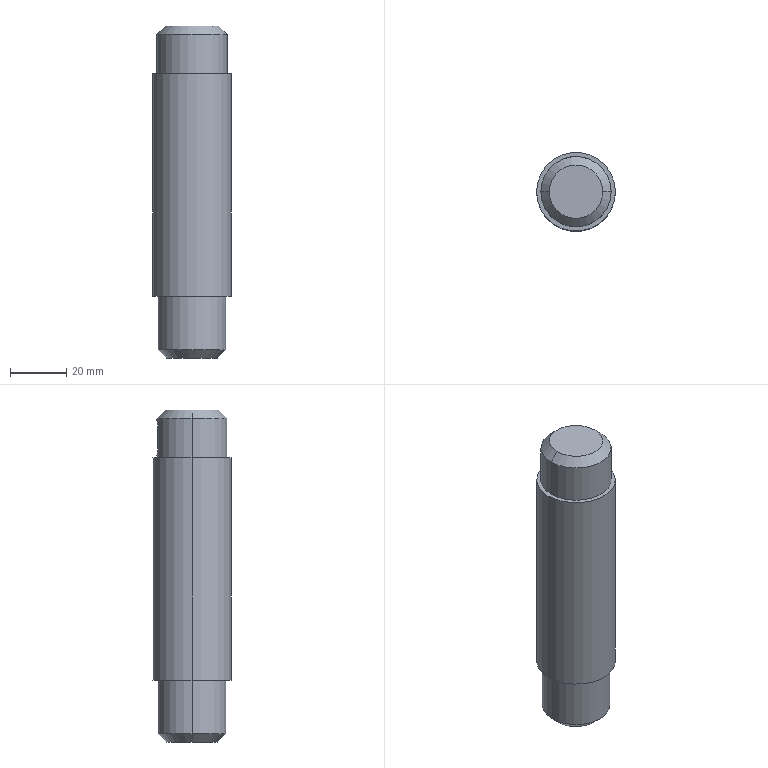Part | SolidWorks | features ICE 2, Chamfer 1, Cut 1, Extrusion 1, MoveFace 1 | 1 solid | 20 faces | box 28 x 28 x 118 mm | volume 66131 mm3 | cylinder 9 | plane 7 | cone 4 | commonest cylinder face diameters 5 x3 24 x2 25 x2 28 x2
STEP:
#1=CARTESIAN_POINT('',(0.,9.5,92.7));
#2=VERTEX_POINT('',#1);
#3=CARTESIAN_POINT('',(2.5,9.5,90.2));
#4=VERTEX_POINT('',#3);
#5=CARTESIAN_POINT('',(0.,9.5,90.2));
#6=DIRECTION('',(0.,1.,0.));
#7=DIRECTION('',(0.,0.,1.));
#8=AXIS2_PLACEMENT_3D('',#5,#6,#7);
#9=CIRCLE('',#8,2.5);
#10=EDGE_CURVE('',#2,#4,#9,.T.);
#11=ORIENTED_EDGE('',*,*,#10,.F.);
#12=CARTESIAN_POINT('',(0.,12.5,92.7));
#13=VERTEX_POINT('',#12);
#14=CARTESIAN_POINT('',(0.,9.5,92.7));
#15=DIRECTION('',(0.,1.,0.));
#16=VECTOR('',#15,1000.);
#17=LINE('',#14,#16);
#18=EDGE_CURVE('',#2,#13,#17,.T.);
#19=ORIENTED_EDGE('',*,*,#18,.T.);
#20=CARTESIAN_POINT('',(2.5,12.247,90.2));
#21=VERTEX_POINT('',#20);
#22=CARTESIAN_POINT('',(0.,12.5,92.7));
#23=CARTESIAN_POINT('',(0.1634,12.5,92.7));
#24=CARTESIAN_POINT('',(0.3294,12.497,92.684));
#25=CARTESIAN_POINT('',(0.6501,12.484,92.62));
#26=CARTESIAN_POINT('',(0.806,12.475,92.572));
#27=CARTESIAN_POINT('',(1.109,12.452,92.447));
#28=CARTESIAN_POINT('',(1.255,12.438,92.368));
#29=CARTESIAN_POINT('',(1.525,12.407,92.188));
#30=CARTESIAN_POINT('',(1.651,12.391,92.084));
#31=CARTESIAN_POINT('',(1.884,12.358,91.852));
#32=CARTESIAN_POINT('',(1.987,12.341,91.726));
#33=CARTESIAN_POINT('',(2.168,12.311,91.456));
#34=CARTESIAN_POINT('',(2.246,12.297,91.31));
#35=CARTESIAN_POINT('',(2.371,12.273,91.008));
#36=CARTESIAN_POINT('',(2.419,12.264,90.852));
#37=CARTESIAN_POINT('',(2.483,12.251,90.531));
#38=CARTESIAN_POINT('',(2.5,12.247,90.366));
#39=CARTESIAN_POINT('',(2.5,12.247,90.2));
#40=B_SPLINE_CURVE_WITH_KNOTS('',3,(#22,#23,#24,#25,#26,#27,#28,#29,#30,#31,#32,#33,#34,#35,#36,#37,#38,#39),.UNSPECIFIED.,.F.,.F.,(4,2,2,2,2,2,2,2,4),(0.003919,0.004408,0.004898,0.005387,0.005876,0.006366,0.006855,0.007344,0.007834),.UNSPECIFIED.);
#41=EDGE_CURVE('',#13,#21,#40,.T.);
#42=ORIENTED_EDGE('',*,*,#41,.T.);
#43=CARTESIAN_POINT('',(2.5,9.5,90.2));
#44=DIRECTION('',(0.,1.,0.));
#45=VECTOR('',#44,1000.);
#46=LINE('',#43,#45);
#47=EDGE_CURVE('',#4,#21,#46,.T.);
#48=ORIENTED_EDGE('',*,*,#47,.F.);
#49=EDGE_LOOP('',(#11,#19,#42,#48));
#50=FACE_OUTER_BOUND('',#49,.T.);
#51=CARTESIAN_POINT('',(0.,9.5,90.2));
#52=DIRECTION('',(0.,1.,0.));
#53=DIRECTION('',(0.,0.,1.));
#54=AXIS2_PLACEMENT_3D('',#51,#52,#53);
#55=CYLINDRICAL_SURFACE('',#54,2.5);
#56=ADVANCED_FACE('',(#50),#55,.F.);
#57=CARTESIAN_POINT('',(9.5,0.,96.));
#58=VERTEX_POINT('',#57);
#59=CARTESIAN_POINT('',(-9.5,0.,96.));
#60=VERTEX_POINT('',#59);
#61=CARTESIAN_POINT('',(0.,0.,96.));
#62=DIRECTION('',(0.,0.,1.));
#63=DIRECTION('',(1.,0.,0.));
#64=AXIS2_PLACEMENT_3D('',#61,#62,#63);
#65=CIRCLE('',#64,9.5);
#66=EDGE_CURVE('',#58,#60,#65,.T.);
#67=ORIENTED_EDGE('',*,*,#66,.F.);
#68=CARTESIAN_POINT('',(12.5,0.,93.));
#69=VERTEX_POINT('',#68);
#70=CARTESIAN_POINT('',(9.5,0.,96.));
#71=DIRECTION('',(0.7071,0.,-0.7071));
#72=VECTOR('',#71,1000.);
#73=LINE('',#70,#72);
#74=EDGE_CURVE('',#58,#69,#73,.T.);
#75=ORIENTED_EDGE('',*,*,#74,.T.);
#76=CARTESIAN_POINT('',(-12.5,0.,93.));
#77=VERTEX_POINT('',#76);
#78=CARTESIAN_POINT('',(0.,0.,93.));
#79=DIRECTION('',(0.,0.,-1.));
#80=DIRECTION('',(1.,0.,0.));
#81=AXIS2_PLACEMENT_3D('',#78,#79,#80);
#82=CIRCLE('',#81,12.5);
#83=EDGE_CURVE('',#77,#69,#82,.T.);
#84=ORIENTED_EDGE('',*,*,#83,.F.);
#85=CARTESIAN_POINT('',(-9.5,0.,96.));
#86=DIRECTION('',(-0.7071,0.,-0.7071));
#87=VECTOR('',#86,1000.);
#88=LINE('',#85,#87);
#89=EDGE_CURVE('',#60,#77,#88,.T.);
#90=ORIENTED_EDGE('',*,*,#89,.F.);
#91=EDGE_LOOP('',(#67,#75,#84,#90));
#92=FACE_OUTER_BOUND('',#91,.T.);
#93=CARTESIAN_POINT('',(0.,0.,96.));
#94=DIRECTION('',(0.,0.,-1.));
#95=DIRECTION('',(-1.,0.,0.));
#96=AXIS2_PLACEMENT_3D('',#93,#94,#95);
#97=CONICAL_SURFACE('',#96,9.5,0.7854);
#98=ADVANCED_FACE('',(#92),#97,.T.);
#99=CARTESIAN_POINT('',(-9.,0.,-22.));
#100=VERTEX_POINT('',#99);
#101=CARTESIAN_POINT('',(9.,0.,-22.));
#102=VERTEX_POINT('',#101);
#103=CARTESIAN_POINT('',(0.,0.,-22.));
#104=DIRECTION('',(0.,0.,-1.));
#105=DIRECTION('',(1.,0.,0.));
#106=AXIS2_PLACEMENT_3D('',#103,#104,#105);
#107=CIRCLE('',#106,9.);
#108=EDGE_CURVE('',#100,#102,#107,.T.);
#109=ORIENTED_EDGE('',*,*,#108,.F.);
#110=CARTESIAN_POINT('',(-12.,0.,-19.));
#111=VERTEX_POINT('',#110);
#112=CARTESIAN_POINT('',(-12.,0.,-19.));
#113=DIRECTION('',(-0.7071,0.,0.7071));
#114=VECTOR('',#113,1000.);
#115=LINE('',#112,#114);
#116=EDGE_CURVE('',#100,#111,#115,.T.);
#117=ORIENTED_EDGE('',*,*,#116,.T.);
#118=CARTESIAN_POINT('',(12.,0.,-19.));
#119=VERTEX_POINT('',#118);
#120=CARTESIAN_POINT('',(0.,0.,-19.));
#121=DIRECTION('',(0.,0.,1.));
#122=DIRECTION('',(1.,0.,0.));
#123=AXIS2_PLACEMENT_3D('',#120,#121,#122);
#124=CIRCLE('',#123,12.);
#125=EDGE_CURVE('',#119,#111,#124,.T.);
#126=ORIENTED_EDGE('',*,*,#125,.F.);
#127=CARTESIAN_POINT('',(12.,0.,-19.));
#128=DIRECTION('',(0.7071,0.,0.7071));
#129=VECTOR('',#128,1000.);
#130=LINE('',#127,#129);
#131=EDGE_CURVE('',#102,#119,#130,.T.);
#132=ORIENTED_EDGE('',*,*,#131,.F.);
#133=EDGE_LOOP('',(#109,#117,#126,#132));
#134=FACE_OUTER_BOUND('',#133,.T.);
#135=CARTESIAN_POINT('',(0.,0.,-19.));
#136=DIRECTION('',(0.,0.,1.));
#137=DIRECTION('',(1.,0.,0.));
#138=AXIS2_PLACEMENT_3D('',#135,#136,#137);
#139=CONICAL_SURFACE('',#138,12.,0.7854);
#140=ADVANCED_FACE('',(#134),#139,.T.);
#141=CARTESIAN_POINT('',(2.5,12.247,82.2));
#142=VERTEX_POINT('',#141);
#143=CARTESIAN_POINT('',(-2.5,12.247,82.2));
#144=VERTEX_POINT('',#143);
#145=CARTESIAN_POINT('',(2.5,12.247,82.2));
#146=CARTESIAN_POINT('',(2.5,12.247,82.034));
#147=CARTESIAN_POINT('',(2.484,12.251,81.872));
#148=CARTESIAN_POINT('',(2.42,12.264,81.552));
#149=CARTESIAN_POINT('',(2.372,12.273,81.393));
#150=CARTESIAN_POINT('',(2.246,12.297,81.09));
#151=CARTESIAN_POINT('',(2.169,12.311,80.947));
#152=CARTESIAN_POINT('',(1.988,12.341,80.675));
#153=CARTESIAN_POINT('',(1.883,12.358,80.547));
#154=CARTESIAN_POINT('',(1.538,12.407,80.202));
#155=CARTESIAN_POINT('',(1.26,12.44,80.016));
#156=CARTESIAN_POINT('',(0.8088,12.475,79.829));
#157=CARTESIAN_POINT('',(0.6508,12.484,79.781));
#158=CARTESIAN_POINT('',(0.328,12.497,79.716));
#159=CARTESIAN_POINT('',(0.1655,12.5,79.7));
#160=CARTESIAN_POINT('',(-0.1614,12.5,79.7));
#161=CARTESIAN_POINT('',(-0.3276,12.497,79.716));
#162=CARTESIAN_POINT('',(-0.6485,12.484,79.78));
#163=CARTESIAN_POINT('',(-0.8045,12.475,79.827));
#164=CARTESIAN_POINT('',(-1.108,12.452,79.953));
#165=CARTESIAN_POINT('',(-1.253,12.438,80.031));
#166=CARTESIAN_POINT('',(-1.524,12.408,80.211));
#167=CARTESIAN_POINT('',(-1.651,12.391,80.315));
#168=CARTESIAN_POINT('',(-1.883,12.358,80.547));
#169=CARTESIAN_POINT('',(-1.986,12.342,80.673));
#170=CARTESIAN_POINT('',(-2.167,12.311,80.943));
#171=CARTESIAN_POINT('',(-2.246,12.297,81.09));
#172=CARTESIAN_POINT('',(-2.371,12.273,81.392));
#173=CARTESIAN_POINT('',(-2.419,12.264,81.547));
#174=CARTESIAN_POINT('',(-2.483,12.251,81.869));
#175=CARTESIAN_POINT('',(-2.5,12.247,82.034));
#176=CARTESIAN_POINT('',(-2.5,12.247,82.2));
#177=B_SPLINE_CURVE_WITH_KNOTS('',3,(#145,#146,#147,#148,#149,#150,#151,#152,#153,#154,#155,#156,#157,#158,#159,#160,#161,#162,#163,#164,#165,#166,#167,#168,#169,#170,#171,#172,#173,#174,#175,#176),.UNSPECIFIED.,.F.,.F.,(4,2,2,2,2,2,2,2,2,2,2,2,2,2,2,4),(0.,0.0004896,0.0009792,0.001469,0.001958,0.002938,0.003427,0.003917,0.004407,0.004896,0.005386,0.005875,0.006365,0.006855,0.007344,0.007834),.UNSPECIFIED.);
#178=EDGE_CURVE('',#142,#144,#177,.T.);
#179=ORIENTED_EDGE('',*,*,#178,.F.);
#180=CARTESIAN_POINT('',(2.5,12.247,30.));
#181=DIRECTION('',(0.,0.,-1.));
#182=VECTOR('',#181,1000.);
#183=LINE('',#180,#182);
#184=EDGE_CURVE('',#21,#142,#183,.T.);
#185=ORIENTED_EDGE('',*,*,#184,.F.);
#186=ORIENTED_EDGE('',*,*,#41,.F.);
#187=CARTESIAN_POINT('',(-2.5,12.247,90.2));
#188=VERTEX_POINT('',#187);
#189=CARTESIAN_POINT('',(-2.5,12.247,90.2));
#190=CARTESIAN_POINT('',(-2.5,12.247,90.366));
#191=CARTESIAN_POINT('',(-2.484,12.251,90.528));
#192=CARTESIAN_POINT('',(-2.42,12.264,90.849));
#193=CARTESIAN_POINT('',(-2.372,12.273,91.008));
#194=CARTESIAN_POINT('',(-2.246,12.297,91.31));
#195=CARTESIAN_POINT('',(-2.169,12.311,91.454));
#196=CARTESIAN_POINT('',(-1.987,12.341,91.725));
#197=CARTESIAN_POINT('',(-1.882,12.358,91.854));
#198=CARTESIAN_POINT('',(-1.537,12.407,92.198));
#199=CARTESIAN_POINT('',(-1.258,12.44,92.385));
#200=CARTESIAN_POINT('',(-0.8073,12.475,92.572));
#201=CARTESIAN_POINT('',(-0.6491,12.484,92.62));
#202=CARTESIAN_POINT('',(-0.3261,12.497,92.684));
#203=CARTESIAN_POINT('',(-0.1636,12.5,92.7));
#204=CARTESIAN_POINT('',(0.,12.5,92.7));
#205=B_SPLINE_CURVE_WITH_KNOTS('',3,(#189,#190,#191,#192,#193,#194,#195,#196,#197,#198,#199,#200,#201,#202,#203,#204),.UNSPECIFIED.,.F.,.F.,(4,2,2,2,2,2,2,4),(0.,0.0004899,0.0009797,0.00147,0.001959,0.002939,0.003429,0.003919),.UNSPECIFIED.);
#206=EDGE_CURVE('',#188,#13,#205,.T.);
#207=ORIENTED_EDGE('',*,*,#206,.F.);
#208=CARTESIAN_POINT('',(-2.5,12.247,30.));
#209=DIRECTION('',(0.,0.,1.));
#210=VECTOR('',#209,1000.);
#211=LINE('',#208,#210);
#212=EDGE_CURVE('',#144,#188,#211,.T.);
#213=ORIENTED_EDGE('',*,*,#212,.F.);
#214=EDGE_LOOP('',(#179,#185,#186,#207,#213));
#215=FACE_BOUND('',#214,.T.);
#216=CARTESIAN_POINT('',(12.5,0.,79.));
#217=VERTEX_POINT('',#216);
#218=CARTESIAN_POINT('',(-12.5,0.,79.));
#219=VERTEX_POINT('',#218);
#220=CARTESIAN_POINT('',(0.,0.,79.));
#221=DIRECTION('',(0.,0.,1.));
#222=DIRECTION('',(1.,0.,0.));
#223=AXIS2_PLACEMENT_3D('',#220,#221,#222);
#224=CIRCLE('',#223,12.5);
#225=EDGE_CURVE('',#217,#219,#224,.T.);
#226=ORIENTED_EDGE('',*,*,#225,.T.);
#227=CARTESIAN_POINT('',(-12.5,0.,30.));
#228=DIRECTION('',(0.,0.,1.));
#229=VECTOR('',#228,1000.);
#230=LINE('',#227,#229);
#231=EDGE_CURVE('',#219,#77,#230,.T.);
#232=ORIENTED_EDGE('',*,*,#231,.T.);
#233=ORIENTED_EDGE('',*,*,#83,.T.);
#234=CARTESIAN_POINT('',(12.5,0.,30.));
#235=DIRECTION('',(0.,0.,1.));
#236=VECTOR('',#235,1000.);
#237=LINE('',#234,#236);
#238=EDGE_CURVE('',#217,#69,#237,.T.);
#239=ORIENTED_EDGE('',*,*,#238,.F.);
#240=EDGE_LOOP('',(#226,#232,#233,#239));
#241=FACE_OUTER_BOUND('',#240,.T.);
#242=CARTESIAN_POINT('',(0.,0.,30.));
#243=DIRECTION('',(0.,0.,1.));
#244=DIRECTION('',(1.,0.,0.));
#245=AXIS2_PLACEMENT_3D('',#242,#243,#244);
#246=CYLINDRICAL_SURFACE('',#245,12.5);
#247=ADVANCED_FACE('',(#215,#241),#246,.T.);
#248=ORIENTED_EDGE('',*,*,#125,.T.);
#249=CARTESIAN_POINT('',(-12.,0.,0.));
#250=VERTEX_POINT('',#249);
#251=CARTESIAN_POINT('',(-12.,0.,-22.));
#252=DIRECTION('',(0.,0.,1.));
#253=VECTOR('',#252,1000.);
#254=LINE('',#251,#253);
#255=EDGE_CURVE('',#111,#250,#254,.T.);
#256=ORIENTED_EDGE('',*,*,#255,.T.);
#257=CARTESIAN_POINT('',(12.,0.,0.));
#258=VERTEX_POINT('',#257);
#259=CARTESIAN_POINT('',(0.,0.,0.));
#260=DIRECTION('',(0.,0.,1.));
#261=DIRECTION('',(1.,0.,0.));
#262=AXIS2_PLACEMENT_3D('',#259,#260,#261);
#263=CIRCLE('',#262,12.);
#264=EDGE_CURVE('',#258,#250,#263,.T.);
#265=ORIENTED_EDGE('',*,*,#264,.F.);
#266=CARTESIAN_POINT('',(12.,0.,-22.));
#267=DIRECTION('',(0.,0.,1.));
#268=VECTOR('',#267,1000.);
#269=LINE('',#266,#268);
#270=EDGE_CURVE('',#119,#258,#269,.T.);
#271=ORIENTED_EDGE('',*,*,#270,.F.);
#272=EDGE_LOOP('',(#248,#256,#265,#271));
#273=FACE_OUTER_BOUND('',#272,.T.);
#274=CARTESIAN_POINT('',(0.,0.,-22.));
#275=DIRECTION('',(0.,0.,1.));
#276=DIRECTION('',(1.,0.,0.));
#277=AXIS2_PLACEMENT_3D('',#274,#275,#276);
#278=CYLINDRICAL_SURFACE('',#277,12.);
#279=ADVANCED_FACE('',(#273),#278,.T.);
#280=CARTESIAN_POINT('',(14.,0.,79.));
#281=VERTEX_POINT('',#280);
#282=CARTESIAN_POINT('',(-14.,0.,79.));
#283=VERTEX_POINT('',#282);
#284=CARTESIAN_POINT('',(0.,0.,79.));
#285=DIRECTION('',(0.,0.,1.));
#286=DIRECTION('',(1.,0.,0.));
#287=AXIS2_PLACEMENT_3D('',#284,#285,#286);
#288=CIRCLE('',#287,14.);
#289=EDGE_CURVE('',#281,#283,#288,.T.);
#290=ORIENTED_EDGE('',*,*,#289,.F.);
#291=CARTESIAN_POINT('',(14.,0.,0.));
#292=VERTEX_POINT('',#291);
#293=CARTESIAN_POINT('',(14.,0.,96.));
#294=DIRECTION('',(0.,0.,-1.));
#295=VECTOR('',#294,1000.);
#296=LINE('',#293,#295);
#297=EDGE_CURVE('',#281,#292,#296,.T.);
#298=ORIENTED_EDGE('',*,*,#297,.T.);
#299=CARTESIAN_POINT('',(-14.,0.,0.));
#300=VERTEX_POINT('',#299);
#301=CARTESIAN_POINT('',(0.,0.,0.));
#302=DIRECTION('',(0.,0.,1.));
#303=DIRECTION('',(1.,0.,0.));
#304=AXIS2_PLACEMENT_3D('',#301,#302,#303);
#305=CIRCLE('',#304,14.);
#306=EDGE_CURVE('',#292,#300,#305,.T.);
#307=ORIENTED_EDGE('',*,*,#306,.T.);
#308=CARTESIAN_POINT('',(-14.,0.,96.));
#309=DIRECTION('',(0.,0.,-1.));
#310=VECTOR('',#309,1000.);
#311=LINE('',#308,#310);
#312=EDGE_CURVE('',#283,#300,#311,.T.);
#313=ORIENTED_EDGE('',*,*,#312,.F.);
#314=EDGE_LOOP('',(#290,#298,#307,#313));
#315=FACE_OUTER_BOUND('',#314,.T.);
#316=CARTESIAN_POINT('',(0.,0.,96.));
#317=DIRECTION('',(0.,0.,-1.));
#318=DIRECTION('',(-1.,0.,0.));
#319=AXIS2_PLACEMENT_3D('',#316,#317,#318);
#320=CYLINDRICAL_SURFACE('',#319,14.);
#321=ADVANCED_FACE('',(#315),#320,.T.);
#322=ORIENTED_EDGE('',*,*,#297,.F.);
#323=CARTESIAN_POINT('',(0.,0.,79.));
#324=DIRECTION('',(0.,0.,1.));
#325=DIRECTION('',(1.,0.,0.));
#326=AXIS2_PLACEMENT_3D('',#323,#324,#325);
#327=CIRCLE('',#326,14.);
#328=EDGE_CURVE('',#283,#281,#327,.T.);
#329=ORIENTED_EDGE('',*,*,#328,.F.);
#330=ORIENTED_EDGE('',*,*,#312,.T.);
#331=CARTESIAN_POINT('',(0.,0.,0.));
#332=DIRECTION('',(0.,0.,1.));
#333=DIRECTION('',(1.,0.,0.));
#334=AXIS2_PLACEMENT_3D('',#331,#332,#333);
#335=CIRCLE('',#334,14.);
#336=EDGE_CURVE('',#300,#292,#335,.T.);
#337=ORIENTED_EDGE('',*,*,#336,.T.);
#338=EDGE_LOOP('',(#322,#329,#330,#337));
#339=FACE_OUTER_BOUND('',#338,.T.);
#340=CARTESIAN_POINT('',(0.,0.,96.));
#341=DIRECTION('',(0.,0.,-1.));
#342=DIRECTION('',(-1.,0.,0.));
#343=AXIS2_PLACEMENT_3D('',#340,#341,#342);
#344=CYLINDRICAL_SURFACE('',#343,14.);
#345=ADVANCED_FACE('',(#339),#344,.T.);
#346=ORIENTED_EDGE('',*,*,#255,.F.);
#347=CARTESIAN_POINT('',(0.,0.,-19.));
#348=DIRECTION('',(0.,0.,1.));
#349=DIRECTION('',(1.,0.,0.));
#350=AXIS2_PLACEMENT_3D('',#347,#348,#349);
#351=CIRCLE('',#350,12.);
#352=EDGE_CURVE('',#111,#119,#351,.T.);
#353=ORIENTED_EDGE('',*,*,#352,.T.);
#354=ORIENTED_EDGE('',*,*,#270,.T.);
#355=CARTESIAN_POINT('',(0.,0.,0.));
#356=DIRECTION('',(0.,0.,1.));
#357=DIRECTION('',(1.,0.,0.));
#358=AXIS2_PLACEMENT_3D('',#355,#356,#357);
#359=CIRCLE('',#358,12.);
#360=EDGE_CURVE('',#250,#258,#359,.T.);
#361=ORIENTED_EDGE('',*,*,#360,.F.);
#362=EDGE_LOOP('',(#346,#353,#354,#361));
#363=FACE_OUTER_BOUND('',#362,.T.);
#364=CARTESIAN_POINT('',(0.,0.,-22.));
#365=DIRECTION('',(0.,0.,1.));
#366=DIRECTION('',(1.,0.,0.));
#367=AXIS2_PLACEMENT_3D('',#364,#365,#366);
#368=CYLINDRICAL_SURFACE('',#367,12.);
#369=ADVANCED_FACE('',(#363),#368,.T.);
#370=CARTESIAN_POINT('',(0.,0.,-22.));
#371=DIRECTION('',(0.,0.,-1.));
#372=DIRECTION('',(1.,0.,0.));
#373=AXIS2_PLACEMENT_3D('',#370,#371,#372);
#374=CIRCLE('',#373,9.);
#375=EDGE_CURVE('',#102,#100,#374,.T.);
#376=ORIENTED_EDGE('',*,*,#375,.T.);
#377=ORIENTED_EDGE('',*,*,#108,.T.);
#378=EDGE_LOOP('',(#376,#377));
#379=FACE_OUTER_BOUND('',#378,.T.);
#380=CARTESIAN_POINT('',(0.,0.,-22.));
#381=DIRECTION('',(0.,0.,1.));
#382=DIRECTION('',(1.,0.,0.));
#383=AXIS2_PLACEMENT_3D('',#380,#381,#382);
#384=PLANE('',#383);
#385=ADVANCED_FACE('',(#379),#384,.F.);
#386=ORIENTED_EDGE('',*,*,#264,.T.);
#387=ORIENTED_EDGE('',*,*,#360,.T.);
#388=EDGE_LOOP('',(#386,#387));
#389=FACE_BOUND('',#388,.T.);
#390=ORIENTED_EDGE('',*,*,#336,.F.);
#391=ORIENTED_EDGE('',*,*,#306,.F.);
#392=EDGE_LOOP('',(#390,#391));
#393=FACE_OUTER_BOUND('',#392,.T.);
#394=CARTESIAN_POINT('',(0.,0.,0.));
#395=DIRECTION('',(0.,0.,1.));
#396=DIRECTION('',(1.,0.,0.));
#397=AXIS2_PLACEMENT_3D('',#394,#395,#396);
#398=PLANE('',#397);
#399=ADVANCED_FACE('',(#389,#393),#398,.F.);
#400=ORIENTED_EDGE('',*,*,#225,.F.);
#401=CARTESIAN_POINT('',(0.,0.,79.));
#402=DIRECTION('',(0.,0.,1.));
#403=DIRECTION('',(1.,0.,0.));
#404=AXIS2_PLACEMENT_3D('',#401,#402,#403);
#405=CIRCLE('',#404,12.5);
#406=EDGE_CURVE('',#219,#217,#405,.T.);
#407=ORIENTED_EDGE('',*,*,#406,.F.);
#408=EDGE_LOOP('',(#400,#407));
#409=FACE_BOUND('',#408,.T.);
#410=ORIENTED_EDGE('',*,*,#328,.T.);
#411=ORIENTED_EDGE('',*,*,#289,.T.);
#412=EDGE_LOOP('',(#410,#411));
#413=FACE_OUTER_BOUND('',#412,.T.);
#414=CARTESIAN_POINT('',(0.,0.,79.));
#415=DIRECTION('',(0.,0.,1.));
#416=DIRECTION('',(1.,0.,0.));
#417=AXIS2_PLACEMENT_3D('',#414,#415,#416);
#418=PLANE('',#417);
#419=ADVANCED_FACE('',(#409,#413),#418,.T.);
#420=ORIENTED_EDGE('',*,*,#231,.F.);
#421=ORIENTED_EDGE('',*,*,#406,.T.);
#422=ORIENTED_EDGE('',*,*,#238,.T.);
#423=CARTESIAN_POINT('',(0.,0.,93.));
#424=DIRECTION('',(0.,0.,-1.));
#425=DIRECTION('',(1.,0.,0.));
#426=AXIS2_PLACEMENT_3D('',#423,#424,#425);
#427=CIRCLE('',#426,12.5);
#428=EDGE_CURVE('',#69,#77,#427,.T.);
#429=ORIENTED_EDGE('',*,*,#428,.T.);
#430=EDGE_LOOP('',(#420,#421,#422,#429));
#431=FACE_OUTER_BOUND('',#430,.T.);
#432=CARTESIAN_POINT('',(0.,0.,30.));
#433=DIRECTION('',(0.,0.,1.));
#434=DIRECTION('',(1.,0.,0.));
#435=AXIS2_PLACEMENT_3D('',#432,#433,#434);
#436=CYLINDRICAL_SURFACE('',#435,12.5);
#437=ADVANCED_FACE('',(#431),#436,.T.);
#438=CARTESIAN_POINT('',(0.,0.,96.));
#439=DIRECTION('',(0.,0.,1.));
#440=DIRECTION('',(1.,0.,0.));
#441=AXIS2_PLACEMENT_3D('',#438,#439,#440);
#442=CIRCLE('',#441,9.5);
#443=EDGE_CURVE('',#60,#58,#442,.T.);
#444=ORIENTED_EDGE('',*,*,#443,.T.);
#445=ORIENTED_EDGE('',*,*,#66,.T.);
#446=EDGE_LOOP('',(#444,#445));
#447=FACE_OUTER_BOUND('',#446,.T.);
#448=CARTESIAN_POINT('',(0.,0.,96.));
#449=DIRECTION('',(0.,0.,1.));
#450=DIRECTION('',(1.,0.,0.));
#451=AXIS2_PLACEMENT_3D('',#448,#449,#450);
#452=PLANE('',#451);
#453=ADVANCED_FACE('',(#447),#452,.T.);
#454=ORIENTED_EDGE('',*,*,#116,.F.);
#455=ORIENTED_EDGE('',*,*,#375,.F.);
#456=ORIENTED_EDGE('',*,*,#131,.T.);
#457=ORIENTED_EDGE('',*,*,#352,.F.);
#458=EDGE_LOOP('',(#454,#455,#456,#457));
#459=FACE_OUTER_BOUND('',#458,.T.);
#460=CARTESIAN_POINT('',(0.,0.,-19.));
#461=DIRECTION('',(0.,0.,1.));
#462=DIRECTION('',(1.,0.,0.));
#463=AXIS2_PLACEMENT_3D('',#460,#461,#462);
#464=CONICAL_SURFACE('',#463,12.,0.7854);
#465=ADVANCED_FACE('',(#459),#464,.T.);
#466=ORIENTED_EDGE('',*,*,#74,.F.);
#467=ORIENTED_EDGE('',*,*,#443,.F.);
#468=ORIENTED_EDGE('',*,*,#89,.T.);
#469=ORIENTED_EDGE('',*,*,#428,.F.);
#470=EDGE_LOOP('',(#466,#467,#468,#469));
#471=FACE_OUTER_BOUND('',#470,.T.);
#472=CARTESIAN_POINT('',(0.,0.,96.));
#473=DIRECTION('',(0.,0.,-1.));
#474=DIRECTION('',(-1.,0.,0.));
#475=AXIS2_PLACEMENT_3D('',#472,#473,#474);
#476=CONICAL_SURFACE('',#475,9.5,0.7854);
#477=ADVANCED_FACE('',(#471),#476,.T.);
#478=ORIENTED_EDGE('',*,*,#18,.F.);
#479=CARTESIAN_POINT('',(-2.5,9.5,90.2));
#480=VERTEX_POINT('',#479);
#481=CARTESIAN_POINT('',(0.,9.5,90.2));
#482=DIRECTION('',(0.,1.,0.));
#483=DIRECTION('',(0.,0.,1.));
#484=AXIS2_PLACEMENT_3D('',#481,#482,#483);
#485=CIRCLE('',#484,2.5);
#486=EDGE_CURVE('',#480,#2,#485,.T.);
#487=ORIENTED_EDGE('',*,*,#486,.F.);
#488=CARTESIAN_POINT('',(-2.5,9.5,90.2));
#489=DIRECTION('',(0.,1.,0.));
#490=VECTOR('',#489,1000.);
#491=LINE('',#488,#490);
#492=EDGE_CURVE('',#480,#188,#491,.T.);
#493=ORIENTED_EDGE('',*,*,#492,.T.);
#494=ORIENTED_EDGE('',*,*,#206,.T.);
#495=EDGE_LOOP('',(#478,#487,#493,#494));
#496=FACE_OUTER_BOUND('',#495,.T.);
#497=CARTESIAN_POINT('',(0.,9.5,90.2));
#498=DIRECTION('',(0.,1.,0.));
#499=DIRECTION('',(0.,0.,1.));
#500=AXIS2_PLACEMENT_3D('',#497,#498,#499);
#501=CYLINDRICAL_SURFACE('',#500,2.5);
#502=ADVANCED_FACE('',(#496),#501,.F.);
#503=ORIENTED_EDGE('',*,*,#212,.T.);
#504=ORIENTED_EDGE('',*,*,#492,.F.);
#505=CARTESIAN_POINT('',(-2.5,9.5,82.2));
#506=VERTEX_POINT('',#505);
#507=CARTESIAN_POINT('',(-2.5,9.5,90.2));
#508=DIRECTION('',(0.,0.,1.));
#509=VECTOR('',#508,1000.);
#510=LINE('',#507,#509);
#511=EDGE_CURVE('',#506,#480,#510,.T.);
#512=ORIENTED_EDGE('',*,*,#511,.F.);
#513=CARTESIAN_POINT('',(-2.5,9.5,82.2));
#514=DIRECTION('',(0.,1.,0.));
#515=VECTOR('',#514,1000.);
#516=LINE('',#513,#515);
#517=EDGE_CURVE('',#506,#144,#516,.T.);
#518=ORIENTED_EDGE('',*,*,#517,.T.);
#519=EDGE_LOOP('',(#503,#504,#512,#518));
#520=FACE_OUTER_BOUND('',#519,.T.);
#521=CARTESIAN_POINT('',(-2.5,9.5,90.2));
#522=DIRECTION('',(-1.,0.,0.));
#523=DIRECTION('',(0.,0.,1.));
#524=AXIS2_PLACEMENT_3D('',#521,#522,#523);
#525=PLANE('',#524);
#526=ADVANCED_FACE('',(#520),#525,.F.);
#527=CARTESIAN_POINT('',(2.5,9.5,82.2));
#528=VERTEX_POINT('',#527);
#529=CARTESIAN_POINT('',(2.5,9.5,82.2));
#530=DIRECTION('',(0.,1.,0.));
#531=VECTOR('',#530,1000.);
#532=LINE('',#529,#531);
#533=EDGE_CURVE('',#528,#142,#532,.T.);
#534=ORIENTED_EDGE('',*,*,#533,.T.);
#535=ORIENTED_EDGE('',*,*,#178,.T.);
#536=ORIENTED_EDGE('',*,*,#517,.F.);
#537=CARTESIAN_POINT('',(0.,9.5,82.2));
#538=DIRECTION('',(0.,1.,0.));
#539=DIRECTION('',(0.,0.,1.));
#540=AXIS2_PLACEMENT_3D('',#537,#538,#539);
#541=CIRCLE('',#540,2.5);
#542=EDGE_CURVE('',#528,#506,#541,.T.);
#543=ORIENTED_EDGE('',*,*,#542,.F.);
#544=EDGE_LOOP('',(#534,#535,#536,#543));
#545=FACE_OUTER_BOUND('',#544,.T.);
#546=CARTESIAN_POINT('',(0.,9.5,82.2));
#547=DIRECTION('',(0.,1.,0.));
#548=DIRECTION('',(0.,0.,1.));
#549=AXIS2_PLACEMENT_3D('',#546,#547,#548);
#550=CYLINDRICAL_SURFACE('',#549,2.5);
#551=ADVANCED_FACE('',(#545),#550,.F.);
#552=ORIENTED_EDGE('',*,*,#184,.T.);
#553=ORIENTED_EDGE('',*,*,#533,.F.);
#554=CARTESIAN_POINT('',(2.5,9.5,90.2));
#555=DIRECTION('',(0.,0.,-1.));
#556=VECTOR('',#555,1000.);
#557=LINE('',#554,#556);
#558=EDGE_CURVE('',#4,#528,#557,.T.);
#559=ORIENTED_EDGE('',*,*,#558,.F.);
#560=ORIENTED_EDGE('',*,*,#47,.T.);
#561=EDGE_LOOP('',(#552,#553,#559,#560));
#562=FACE_OUTER_BOUND('',#561,.T.);
#563=CARTESIAN_POINT('',(2.5,9.5,90.2));
#564=DIRECTION('',(1.,0.,0.));
#565=DIRECTION('',(0.,0.,-1.));
#566=AXIS2_PLACEMENT_3D('',#563,#564,#565);
#567=PLANE('',#566);
#568=ADVANCED_FACE('',(#562),#567,.F.);
#569=ORIENTED_EDGE('',*,*,#486,.T.);
#570=ORIENTED_EDGE('',*,*,#10,.T.);
#571=ORIENTED_EDGE('',*,*,#558,.T.);
#572=ORIENTED_EDGE('',*,*,#542,.T.);
#573=ORIENTED_EDGE('',*,*,#511,.T.);
#574=EDGE_LOOP('',(#569,#570,#571,#572,#573));
#575=FACE_OUTER_BOUND('',#574,.T.);
#576=CARTESIAN_POINT('',(0.,9.5,90.2));
#577=DIRECTION('',(0.,1.,0.));
#578=DIRECTION('',(0.,0.,1.));
#579=AXIS2_PLACEMENT_3D('',#576,#577,#578);
#580=PLANE('',#579);
#581=ADVANCED_FACE('',(#575),#580,.T.);
#582=CLOSED_SHELL('',(#56,#98,#140,#247,#279,#321,#345,#369,#385,#399,#419,#437,#453,#465,#477,#502,#526,#551,#568,#581));
#583=MANIFOLD_SOLID_BREP('',#582);
#584=CARTESIAN_POINT('',(0.,0.,0.));
#585=DIRECTION('',(0.,0.,1.));
#586=DIRECTION('',(1.,0.,0.));
#587=AXIS2_PLACEMENT_3D('',#584,#585,#586);
#588=(LENGTH_UNIT()NAMED_UNIT(*)SI_UNIT(.MILLI.,.METRE.));
#589=UNCERTAINTY_MEASURE_WITH_UNIT(LENGTH_MEASURE(0.00001),#588,'','');
#590=(NAMED_UNIT(*)PLANE_ANGLE_UNIT()SI_UNIT($,.RADIAN.));
#591=(NAMED_UNIT(*)SI_UNIT($,.STERADIAN.)SOLID_ANGLE_UNIT());
#592=(GEOMETRIC_REPRESENTATION_CONTEXT(3)GLOBAL_UNCERTAINTY_ASSIGNED_CONTEXT((#589))GLOBAL_UNIT_ASSIGNED_CONTEXT((#588,#590,#591))REPRESENTATION_CONTEXT('',''));
#593=ADVANCED_BREP_SHAPE_REPRESENTATION('',(#583,#587),#592);